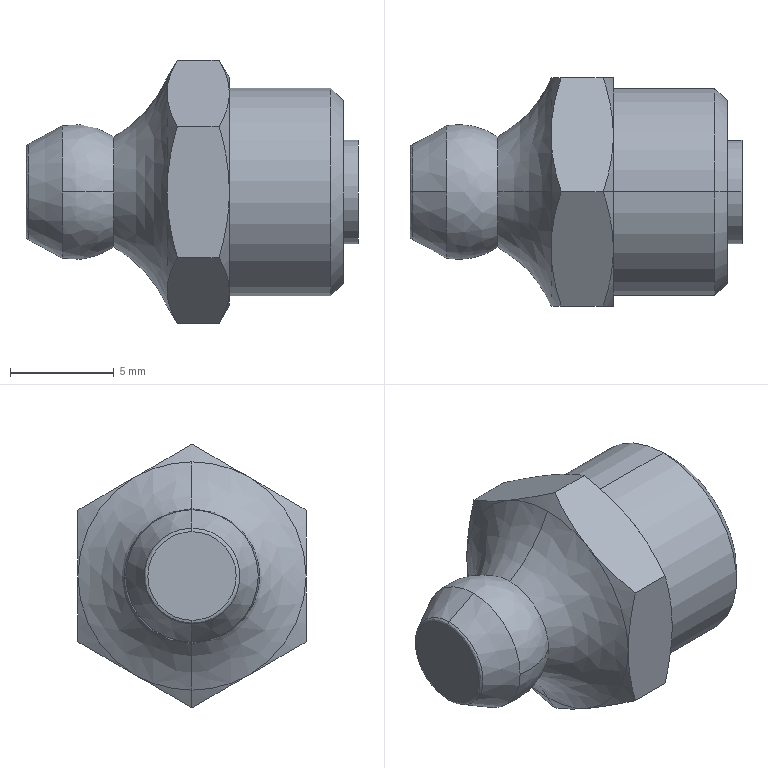Part | SolidWorks | features BaseBody 1 | 1 solid | 38 faces | box 16 x 11 x 12.702 mm | volume 986.989 mm3 | cone 18 | plane 10 | spline 6 | cylinder 4 | commonest cylinder face diameters 5 x2 10 x2
STEP:
#1=CARTESIAN_POINT('',(-5.573,0.,2.65));
#2=VERTEX_POINT('',#1);
#3=CARTESIAN_POINT('',(-5.573,2.65,0.));
#4=VERTEX_POINT('',#3);
#5=CARTESIAN_POINT('',(-5.573,0.,0.));
#6=DIRECTION('',(-1.,0.,0.));
#7=DIRECTION('',(0.,0.,-1.));
#8=AXIS2_PLACEMENT_3D('',#5,#6,#7);
#9=CIRCLE('',#8,2.65);
#10=EDGE_CURVE('',#2,#4,#9,.T.);
#11=ORIENTED_EDGE('',*,*,#10,.F.);
#12=CARTESIAN_POINT('',(-3.,0.,5.5));
#13=VERTEX_POINT('',#12);
#14=CARTESIAN_POINT('',(-8.506,0.,7.885));
#15=DIRECTION('',(0.,-1.,0.));
#16=DIRECTION('',(0.,0.,1.));
#17=AXIS2_PLACEMENT_3D('',#14,#15,#16);
#18=CIRCLE('',#17,6.);
#19=EDGE_CURVE('',#2,#13,#18,.T.);
#20=ORIENTED_EDGE('',*,*,#19,.T.);
#21=CARTESIAN_POINT('',(-3.,2.75,4.763));
#22=VERTEX_POINT('',#21);
#23=CARTESIAN_POINT('',(-3.,0.,0.));
#24=DIRECTION('',(1.,0.,0.));
#25=DIRECTION('',(0.,0.,1.));
#26=AXIS2_PLACEMENT_3D('',#23,#24,#25);
#27=CIRCLE('',#26,5.5);
#28=EDGE_CURVE('',#22,#13,#27,.T.);
#29=ORIENTED_EDGE('',*,*,#28,.F.);
#30=CARTESIAN_POINT('',(-3.,5.5,0.));
#31=VERTEX_POINT('',#30);
#32=CARTESIAN_POINT('',(-3.,0.,0.));
#33=DIRECTION('',(1.,0.,0.));
#34=DIRECTION('',(0.,0.,1.));
#35=AXIS2_PLACEMENT_3D('',#32,#33,#34);
#36=CIRCLE('',#35,5.5);
#37=EDGE_CURVE('',#31,#22,#36,.T.);
#38=ORIENTED_EDGE('',*,*,#37,.F.);
#39=CARTESIAN_POINT('',(-3.,2.75,-4.763));
#40=VERTEX_POINT('',#39);
#41=CARTESIAN_POINT('',(-3.,0.,0.));
#42=DIRECTION('',(1.,0.,0.));
#43=DIRECTION('',(0.,0.,1.));
#44=AXIS2_PLACEMENT_3D('',#41,#42,#43);
#45=CIRCLE('',#44,5.5);
#46=EDGE_CURVE('',#40,#31,#45,.T.);
#47=ORIENTED_EDGE('',*,*,#46,.F.);
#48=CARTESIAN_POINT('',(-3.,0.,-5.5));
#49=VERTEX_POINT('',#48);
#50=CARTESIAN_POINT('',(-3.,0.,0.));
#51=DIRECTION('',(1.,0.,0.));
#52=DIRECTION('',(0.,0.,1.));
#53=AXIS2_PLACEMENT_3D('',#50,#51,#52);
#54=CIRCLE('',#53,5.5);
#55=EDGE_CURVE('',#49,#40,#54,.T.);
#56=ORIENTED_EDGE('',*,*,#55,.F.);
#57=CARTESIAN_POINT('',(-5.573,0.,-2.65));
#58=VERTEX_POINT('',#57);
#59=CARTESIAN_POINT('',(-8.506,0.,-7.885));
#60=DIRECTION('',(0.,1.,0.));
#61=DIRECTION('',(0.,0.,-1.));
#62=AXIS2_PLACEMENT_3D('',#59,#60,#61);
#63=CIRCLE('',#62,6.);
#64=EDGE_CURVE('',#58,#49,#63,.T.);
#65=ORIENTED_EDGE('',*,*,#64,.F.);
#66=CARTESIAN_POINT('',(-5.573,0.,0.));
#67=DIRECTION('',(-1.,0.,0.));
#68=DIRECTION('',(0.,0.,-1.));
#69=AXIS2_PLACEMENT_3D('',#66,#67,#68);
#70=CIRCLE('',#69,2.65);
#71=EDGE_CURVE('',#4,#58,#70,.T.);
#72=ORIENTED_EDGE('',*,*,#71,.F.);
#73=EDGE_LOOP('',(#11,#20,#29,#38,#47,#56,#65,#72));
#74=FACE_OUTER_BOUND('',#73,.T.);
#75=CARTESIAN_POINT('',(-5.573,0.,-2.65));
#76=CARTESIAN_POINT('',(-5.573,5.3,-2.65));
#77=CARTESIAN_POINT('',(-5.573,5.3,2.65));
#78=CARTESIAN_POINT('',(-5.573,0.,2.65));
#79=CARTESIAN_POINT('',(-4.416,0.,-3.298));
#80=CARTESIAN_POINT('',(-4.416,6.597,-3.298));
#81=CARTESIAN_POINT('',(-4.416,6.597,3.298));
#82=CARTESIAN_POINT('',(-4.416,0.,3.298));
#83=CARTESIAN_POINT('',(-3.527,0.,-4.283));
#84=CARTESIAN_POINT('',(-3.527,8.566,-4.283));
#85=CARTESIAN_POINT('',(-3.527,8.566,4.283));
#86=CARTESIAN_POINT('',(-3.527,0.,4.283));
#87=CARTESIAN_POINT('',(-3.,0.,-5.5));
#88=CARTESIAN_POINT('',(-3.,11.,-5.5));
#89=CARTESIAN_POINT('',(-3.,11.,5.5));
#90=CARTESIAN_POINT('',(-3.,0.,5.5));
#91=(BOUNDED_SURFACE()B_SPLINE_SURFACE(3,3,((#75,#76,#77,#78),(#79,#80,#81,#82),(#83,#84,#85,#86),(#87,#88,#89,#90)),.UNSPECIFIED.,.F.,.F.,.T.)B_SPLINE_SURFACE_WITH_KNOTS((4,4),(4,4),(0.,1.),(0.,1.),.UNSPECIFIED.)GEOMETRIC_REPRESENTATION_ITEM()RATIONAL_B_SPLINE_SURFACE(((1.,0.3333,0.3333,1.),(0.9649,0.3216,0.3216,0.9649),(0.9649,0.3216,0.3216,0.9649),(1.,0.3333,0.3333,1.)))REPRESENTATION_ITEM('')SURFACE());
#92=ADVANCED_FACE('',(#74),#91,.F.);
#93=ORIENTED_EDGE('',*,*,#71,.T.);
#94=CARTESIAN_POINT('',(-5.573,-2.65,0.));
#95=VERTEX_POINT('',#94);
#96=CARTESIAN_POINT('',(-5.573,0.,0.));
#97=DIRECTION('',(-1.,0.,0.));
#98=DIRECTION('',(0.,0.,-1.));
#99=AXIS2_PLACEMENT_3D('',#96,#97,#98);
#100=CIRCLE('',#99,2.65);
#101=EDGE_CURVE('',#58,#95,#100,.T.);
#102=ORIENTED_EDGE('',*,*,#101,.T.);
#103=CARTESIAN_POINT('',(-8.055,-3.194,0.));
#104=VERTEX_POINT('',#103);
#105=CARTESIAN_POINT('',(-7.455,0.,0.));
#106=DIRECTION('',(0.,0.,-1.));
#107=DIRECTION('',(1.,0.,0.));
#108=AXIS2_PLACEMENT_3D('',#105,#106,#107);
#109=CIRCLE('',#108,3.25);
#110=EDGE_CURVE('',#95,#104,#109,.T.);
#111=ORIENTED_EDGE('',*,*,#110,.T.);
#112=CARTESIAN_POINT('',(-8.055,0.,-3.194));
#113=VERTEX_POINT('',#112);
#114=CARTESIAN_POINT('',(-8.055,0.,0.));
#115=DIRECTION('',(1.,0.,0.));
#116=DIRECTION('',(0.,1.,0.));
#117=AXIS2_PLACEMENT_3D('',#114,#115,#116);
#118=CIRCLE('',#117,3.194);
#119=EDGE_CURVE('',#104,#113,#118,.T.);
#120=ORIENTED_EDGE('',*,*,#119,.T.);
#121=CARTESIAN_POINT('',(-8.055,3.194,0.));
#122=VERTEX_POINT('',#121);
#123=CARTESIAN_POINT('',(-8.055,0.,0.));
#124=DIRECTION('',(1.,0.,0.));
#125=DIRECTION('',(0.,1.,0.));
#126=AXIS2_PLACEMENT_3D('',#123,#124,#125);
#127=CIRCLE('',#126,3.194);
#128=EDGE_CURVE('',#113,#122,#127,.T.);
#129=ORIENTED_EDGE('',*,*,#128,.T.);
#130=CARTESIAN_POINT('',(-7.455,0.,0.));
#131=DIRECTION('',(0.,0.,1.));
#132=DIRECTION('',(1.,0.,0.));
#133=AXIS2_PLACEMENT_3D('',#130,#131,#132);
#134=CIRCLE('',#133,3.25);
#135=EDGE_CURVE('',#4,#122,#134,.T.);
#136=ORIENTED_EDGE('',*,*,#135,.F.);
#137=EDGE_LOOP('',(#93,#102,#111,#120,#129,#136));
#138=FACE_OUTER_BOUND('',#137,.T.);
#139=CARTESIAN_POINT('',(-5.573,-2.65,0.));
#140=CARTESIAN_POINT('',(-5.573,-2.65,-5.3));
#141=CARTESIAN_POINT('',(-5.573,2.65,-5.3));
#142=CARTESIAN_POINT('',(-5.573,2.65,0.));
#143=CARTESIAN_POINT('',(-6.302,-3.168,0.));
#144=CARTESIAN_POINT('',(-6.302,-3.168,-6.335));
#145=CARTESIAN_POINT('',(-6.302,3.168,-6.335));
#146=CARTESIAN_POINT('',(-6.302,3.168,0.));
#147=CARTESIAN_POINT('',(-7.176,-3.359,0.));
#148=CARTESIAN_POINT('',(-7.176,-3.359,-6.718));
#149=CARTESIAN_POINT('',(-7.176,3.359,-6.718));
#150=CARTESIAN_POINT('',(-7.176,3.359,0.));
#151=CARTESIAN_POINT('',(-8.055,-3.194,0.));
#152=CARTESIAN_POINT('',(-8.055,-3.194,-6.388));
#153=CARTESIAN_POINT('',(-8.055,3.194,-6.388));
#154=CARTESIAN_POINT('',(-8.055,3.194,0.));
#155=(BOUNDED_SURFACE()B_SPLINE_SURFACE(3,3,((#139,#140,#141,#142),(#143,#144,#145,#146),(#147,#148,#149,#150),(#151,#152,#153,#154)),.UNSPECIFIED.,.F.,.F.,.F.)B_SPLINE_SURFACE_WITH_KNOTS((4,4),(4,4),(0.,1.),(0.,1.),.UNSPECIFIED.)GEOMETRIC_REPRESENTATION_ITEM()RATIONAL_B_SPLINE_SURFACE(((1.,0.3333,0.3333,1.),(0.947,0.3157,0.3157,0.947),(0.947,0.3157,0.3157,0.947),(1.,0.3333,0.3333,1.)))REPRESENTATION_ITEM('')SURFACE());
#156=ADVANCED_FACE('',(#138),#155,.T.);
#157=CARTESIAN_POINT('',(-9.695,0.,2.307));
#158=VERTEX_POINT('',#157);
#159=CARTESIAN_POINT('',(-9.695,0.,-2.307));
#160=VERTEX_POINT('',#159);
#161=CARTESIAN_POINT('',(-9.695,0.,0.));
#162=DIRECTION('',(1.,0.,0.));
#163=DIRECTION('',(0.,1.,0.));
#164=AXIS2_PLACEMENT_3D('',#161,#162,#163);
#165=CIRCLE('',#164,2.307);
#166=EDGE_CURVE('',#158,#160,#165,.T.);
#167=ORIENTED_EDGE('',*,*,#166,.F.);
#168=CARTESIAN_POINT('',(-9.8,0.,2.131));
#169=VERTEX_POINT('',#168);
#170=CARTESIAN_POINT('',(-9.6,0.,2.131));
#171=DIRECTION('',(0.,-1.,0.));
#172=DIRECTION('',(0.,0.,1.));
#173=AXIS2_PLACEMENT_3D('',#170,#171,#172);
#174=CIRCLE('',#173,0.2);
#175=EDGE_CURVE('',#158,#169,#174,.T.);
#176=ORIENTED_EDGE('',*,*,#175,.T.);
#177=CARTESIAN_POINT('',(-9.8,0.,-2.131));
#178=VERTEX_POINT('',#177);
#179=CARTESIAN_POINT('',(-9.8,0.,2.131));
#180=CARTESIAN_POINT('',(-9.8,-4.262,2.131));
#181=CARTESIAN_POINT('',(-9.8,-4.262,-2.131));
#182=CARTESIAN_POINT('',(-9.8,0.,-2.131));
#183=(BOUNDED_CURVE()B_SPLINE_CURVE(3,(#179,#180,#181,#182),.UNSPECIFIED.,.F.,.T.)B_SPLINE_CURVE_WITH_KNOTS((4,4),(0.25,0.75),.UNSPECIFIED.)CURVE()GEOMETRIC_REPRESENTATION_ITEM()RATIONAL_B_SPLINE_CURVE((1.,0.3333,0.3333,1.))REPRESENTATION_ITEM(''));
#184=EDGE_CURVE('',#169,#178,#183,.T.);
#185=ORIENTED_EDGE('',*,*,#184,.T.);
#186=CARTESIAN_POINT('',(-9.6,0.,-2.131));
#187=DIRECTION('',(0.,1.,0.));
#188=DIRECTION('',(0.,0.,-1.));
#189=AXIS2_PLACEMENT_3D('',#186,#187,#188);
#190=CIRCLE('',#189,0.2);
#191=EDGE_CURVE('',#160,#178,#190,.T.);
#192=ORIENTED_EDGE('',*,*,#191,.F.);
#193=EDGE_LOOP('',(#167,#176,#185,#192));
#194=FACE_OUTER_BOUND('',#193,.T.);
#195=CARTESIAN_POINT('',(-9.695,0.,2.307));
#196=CARTESIAN_POINT('',(-9.695,-4.613,2.307));
#197=CARTESIAN_POINT('',(-9.695,-4.613,-2.307));
#198=CARTESIAN_POINT('',(-9.695,0.,-2.307));
#199=CARTESIAN_POINT('',(-9.761,0.,2.271));
#200=CARTESIAN_POINT('',(-9.761,-4.542,2.271));
#201=CARTESIAN_POINT('',(-9.761,-4.542,-2.271));
#202=CARTESIAN_POINT('',(-9.761,0.,-2.271));
#203=CARTESIAN_POINT('',(-9.8,0.,2.206));
#204=CARTESIAN_POINT('',(-9.8,-4.412,2.206));
#205=CARTESIAN_POINT('',(-9.8,-4.412,-2.206));
#206=CARTESIAN_POINT('',(-9.8,0.,-2.206));
#207=CARTESIAN_POINT('',(-9.8,0.,2.131));
#208=CARTESIAN_POINT('',(-9.8,-4.262,2.131));
#209=CARTESIAN_POINT('',(-9.8,-4.262,-2.131));
#210=CARTESIAN_POINT('',(-9.8,0.,-2.131));
#211=(BOUNDED_SURFACE()B_SPLINE_SURFACE(3,3,((#195,#196,#197,#198),(#199,#200,#201,#202),(#203,#204,#205,#206),(#207,#208,#209,#210)),.UNSPECIFIED.,.F.,.F.,.F.)B_SPLINE_SURFACE_WITH_KNOTS((4,4),(4,4),(0.,1.),(0.,1.),.UNSPECIFIED.)GEOMETRIC_REPRESENTATION_ITEM()RATIONAL_B_SPLINE_SURFACE(((1.,0.3333,0.3333,1.),(0.906,0.302,0.302,0.906),(0.906,0.302,0.302,0.906),(1.,0.3333,0.3333,1.)))REPRESENTATION_ITEM('')SURFACE());
#212=ADVANCED_FACE('',(#194),#211,.T.);
#213=CARTESIAN_POINT('',(0.,0.,-5.));
#214=VERTEX_POINT('',#213);
#215=CARTESIAN_POINT('',(0.,0.,5.));
#216=VERTEX_POINT('',#215);
#217=CARTESIAN_POINT('',(0.,0.,0.));
#218=DIRECTION('',(1.,0.,0.));
#219=DIRECTION('',(0.,0.,-1.));
#220=AXIS2_PLACEMENT_3D('',#217,#218,#219);
#221=CIRCLE('',#220,5.);
#222=EDGE_CURVE('',#214,#216,#221,.T.);
#223=ORIENTED_EDGE('',*,*,#222,.T.);
#224=CARTESIAN_POINT('',(4.887,0.,5.));
#225=VERTEX_POINT('',#224);
#226=CARTESIAN_POINT('',(2.75,0.,5.));
#227=DIRECTION('',(1.,0.,0.));
#228=VECTOR('',#227,1000.);
#229=LINE('',#226,#228);
#230=EDGE_CURVE('',#216,#225,#229,.T.);
#231=ORIENTED_EDGE('',*,*,#230,.T.);
#232=CARTESIAN_POINT('',(4.887,0.,-5.));
#233=VERTEX_POINT('',#232);
#234=CARTESIAN_POINT('',(4.887,0.,0.));
#235=DIRECTION('',(-1.,0.,0.));
#236=DIRECTION('',(0.,0.,-1.));
#237=AXIS2_PLACEMENT_3D('',#234,#235,#236);
#238=CIRCLE('',#237,5.);
#239=EDGE_CURVE('',#225,#233,#238,.T.);
#240=ORIENTED_EDGE('',*,*,#239,.T.);
#241=CARTESIAN_POINT('',(2.75,0.,-5.));
#242=DIRECTION('',(1.,0.,0.));
#243=VECTOR('',#242,1000.);
#244=LINE('',#241,#243);
#245=EDGE_CURVE('',#214,#233,#244,.T.);
#246=ORIENTED_EDGE('',*,*,#245,.F.);
#247=EDGE_LOOP('',(#223,#231,#240,#246));
#248=FACE_OUTER_BOUND('',#247,.T.);
#249=CARTESIAN_POINT('',(2.75,0.,0.));
#250=DIRECTION('',(1.,0.,0.));
#251=DIRECTION('',(0.,0.,-1.));
#252=AXIS2_PLACEMENT_3D('',#249,#250,#251);
#253=CYLINDRICAL_SURFACE('',#252,5.);
#254=ADVANCED_FACE('',(#248),#253,.T.);
#255=CARTESIAN_POINT('',(5.5,0.,4.387));
#256=VERTEX_POINT('',#255);
#257=CARTESIAN_POINT('',(5.5,0.,-4.387));
#258=VERTEX_POINT('',#257);
#259=CARTESIAN_POINT('',(5.5,0.,0.));
#260=DIRECTION('',(-1.,0.,0.));
#261=DIRECTION('',(0.,0.,1.));
#262=AXIS2_PLACEMENT_3D('',#259,#260,#261);
#263=CIRCLE('',#262,4.387);
#264=EDGE_CURVE('',#256,#258,#263,.T.);
#265=ORIENTED_EDGE('',*,*,#264,.T.);
#266=CARTESIAN_POINT('',(4.887,0.,-5.));
#267=DIRECTION('',(-0.7071,0.,-0.7071));
#268=VECTOR('',#267,1000.);
#269=LINE('',#266,#268);
#270=EDGE_CURVE('',#258,#233,#269,.T.);
#271=ORIENTED_EDGE('',*,*,#270,.T.);
#272=ORIENTED_EDGE('',*,*,#239,.F.);
#273=CARTESIAN_POINT('',(4.887,0.,5.));
#274=DIRECTION('',(-0.7071,0.,0.7071));
#275=VECTOR('',#274,1000.);
#276=LINE('',#273,#275);
#277=EDGE_CURVE('',#256,#225,#276,.T.);
#278=ORIENTED_EDGE('',*,*,#277,.F.);
#279=EDGE_LOOP('',(#265,#271,#272,#278));
#280=FACE_OUTER_BOUND('',#279,.T.);
#281=CARTESIAN_POINT('',(4.887,0.,0.));
#282=DIRECTION('',(-1.,0.,0.));
#283=DIRECTION('',(0.,0.,1.));
#284=AXIS2_PLACEMENT_3D('',#281,#282,#283);
#285=CONICAL_SURFACE('',#284,5.,0.7854);
#286=ADVANCED_FACE('',(#280),#285,.T.);
#287=CARTESIAN_POINT('',(0.,0.,5.5));
#288=VERTEX_POINT('',#287);
#289=CARTESIAN_POINT('',(0.,-2.75,4.763));
#290=VERTEX_POINT('',#289);
#291=CARTESIAN_POINT('',(0.,0.,0.));
#292=DIRECTION('',(1.,0.,0.));
#293=DIRECTION('',(0.,0.,1.));
#294=AXIS2_PLACEMENT_3D('',#291,#292,#293);
#295=CIRCLE('',#294,5.5);
#296=EDGE_CURVE('',#288,#290,#295,.T.);
#297=ORIENTED_EDGE('',*,*,#296,.F.);
#298=CARTESIAN_POINT('',(-0.4912,-0.000000012,6.351));
#299=VERTEX_POINT('',#298);
#300=CARTESIAN_POINT('',(-0.4942,0.,6.356));
#301=DIRECTION('',(-0.5,0.,0.866));
#302=VECTOR('',#301,1000.);
#303=LINE('',#300,#302);
#304=EDGE_CURVE('',#288,#299,#303,.T.);
#305=ORIENTED_EDGE('',*,*,#304,.T.);
#306=CARTESIAN_POINT('',(-0.4912,-0.000000012,6.351));
#307=CARTESIAN_POINT('',(-0.1917,-0.8985,5.832));
#308=CARTESIAN_POINT('',(0.,-1.811,5.305));
#309=CARTESIAN_POINT('',(0.,-2.75,4.763));
#310=B_SPLINE_CURVE_WITH_KNOTS('',3,(#306,#307,#308,#309),.UNSPECIFIED.,.F.,.F.,(4,4),(0.,0.003213),.UNSPECIFIED.);
#311=EDGE_CURVE('',#299,#290,#310,.T.);
#312=ORIENTED_EDGE('',*,*,#311,.T.);
#313=EDGE_LOOP('',(#297,#305,#312));
#314=FACE_OUTER_BOUND('',#313,.T.);
#315=CARTESIAN_POINT('',(-0.4942,0.,0.));
#316=DIRECTION('',(-1.,0.,0.));
#317=DIRECTION('',(0.,0.,1.));
#318=AXIS2_PLACEMENT_3D('',#315,#316,#317);
#319=CONICAL_SURFACE('',#318,6.356,1.047);
#320=ADVANCED_FACE('',(#314),#319,.T.);
#321=CARTESIAN_POINT('',(5.5,0.,2.5));
#322=VERTEX_POINT('',#321);
#323=CARTESIAN_POINT('',(5.5,0.,-2.5));
#324=VERTEX_POINT('',#323);
#325=CARTESIAN_POINT('',(5.5,0.,0.));
#326=DIRECTION('',(-1.,0.,0.));
#327=DIRECTION('',(0.,0.,-1.));
#328=AXIS2_PLACEMENT_3D('',#325,#326,#327);
#329=CIRCLE('',#328,2.5);
#330=EDGE_CURVE('',#322,#324,#329,.T.);
#331=ORIENTED_EDGE('',*,*,#330,.F.);
#332=CARTESIAN_POINT('',(6.2,0.,2.5));
#333=VERTEX_POINT('',#332);
#334=CARTESIAN_POINT('',(5.85,0.,2.5));
#335=DIRECTION('',(1.,0.,0.));
#336=VECTOR('',#335,1000.);
#337=LINE('',#334,#336);
#338=EDGE_CURVE('',#322,#333,#337,.T.);
#339=ORIENTED_EDGE('',*,*,#338,.T.);
#340=CARTESIAN_POINT('',(6.2,0.,-2.5));
#341=VERTEX_POINT('',#340);
#342=CARTESIAN_POINT('',(6.2,0.,0.));
#343=DIRECTION('',(-1.,0.,0.));
#344=DIRECTION('',(0.,0.,-1.));
#345=AXIS2_PLACEMENT_3D('',#342,#343,#344);
#346=CIRCLE('',#345,2.5);
#347=EDGE_CURVE('',#333,#341,#346,.T.);
#348=ORIENTED_EDGE('',*,*,#347,.T.);
#349=CARTESIAN_POINT('',(5.85,0.,-2.5));
#350=DIRECTION('',(1.,0.,0.));
#351=VECTOR('',#350,1000.);
#352=LINE('',#349,#351);
#353=EDGE_CURVE('',#324,#341,#352,.T.);
#354=ORIENTED_EDGE('',*,*,#353,.F.);
#355=EDGE_LOOP('',(#331,#339,#348,#354));
#356=FACE_OUTER_BOUND('',#355,.T.);
#357=CARTESIAN_POINT('',(5.85,0.,0.));
#358=DIRECTION('',(1.,0.,0.));
#359=DIRECTION('',(0.,0.,-1.));
#360=AXIS2_PLACEMENT_3D('',#357,#358,#359);
#361=CYLINDRICAL_SURFACE('',#360,2.5);
#362=ADVANCED_FACE('',(#356),#361,.T.);
#363=CARTESIAN_POINT('',(-3.,-2.75,-4.763));
#364=VERTEX_POINT('',#363);
#365=CARTESIAN_POINT('',(-3.,0.,0.));
#366=DIRECTION('',(1.,0.,0.));
#367=DIRECTION('',(0.,0.,1.));
#368=AXIS2_PLACEMENT_3D('',#365,#366,#367);
#369=CIRCLE('',#368,5.5);
#370=EDGE_CURVE('',#364,#49,#369,.T.);
#371=ORIENTED_EDGE('',*,*,#370,.T.);
#372=CARTESIAN_POINT('',(-2.509,0.,-6.351));
#373=VERTEX_POINT('',#372);
#374=CARTESIAN_POINT('',(-2.506,0.,-6.356));
#375=DIRECTION('',(0.5,0.,-0.866));
#376=VECTOR('',#375,1000.);
#377=LINE('',#374,#376);
#378=EDGE_CURVE('',#49,#373,#377,.T.);
#379=ORIENTED_EDGE('',*,*,#378,.T.);
#380=CARTESIAN_POINT('',(-3.,-2.75,-4.763));
#381=CARTESIAN_POINT('',(-3.,-1.811,-5.305));
#382=CARTESIAN_POINT('',(-2.808,-0.8985,-5.832));
#383=CARTESIAN_POINT('',(-2.509,0.,-6.351));
#384=B_SPLINE_CURVE_WITH_KNOTS('',3,(#380,#381,#382,#383),.UNSPECIFIED.,.F.,.F.,(4,4),(0.,0.003213),.UNSPECIFIED.);
#385=EDGE_CURVE('',#364,#373,#384,.T.);
#386=ORIENTED_EDGE('',*,*,#385,.F.);
#387=EDGE_LOOP('',(#371,#379,#386));
#388=FACE_OUTER_BOUND('',#387,.T.);
#389=CARTESIAN_POINT('',(-2.506,0.,0.));
#390=DIRECTION('',(1.,0.,0.));
#391=DIRECTION('',(0.,0.,-1.));
#392=AXIS2_PLACEMENT_3D('',#389,#390,#391);
#393=CONICAL_SURFACE('',#392,6.356,1.047);
#394=ADVANCED_FACE('',(#388),#393,.T.);
#395=CARTESIAN_POINT('',(-9.695,0.,0.));
#396=DIRECTION('',(1.,0.,0.));
#397=DIRECTION('',(0.,1.,0.));
#398=AXIS2_PLACEMENT_3D('',#395,#396,#397);
#399=CIRCLE('',#398,2.307);
#400=EDGE_CURVE('',#160,#158,#399,.T.);
#401=ORIENTED_EDGE('',*,*,#400,.T.);
#402=CARTESIAN_POINT('',(-8.055,0.,3.194));
#403=VERTEX_POINT('',#402);
#404=CARTESIAN_POINT('',(-8.055,0.,3.194));
#405=DIRECTION('',(0.8795,0.,0.4758));
#406=VECTOR('',#405,1000.);
#407=LINE('',#404,#406);
#408=EDGE_CURVE('',#158,#403,#407,.T.);
#409=ORIENTED_EDGE('',*,*,#408,.T.);
#410=CARTESIAN_POINT('',(-8.055,0.,0.));
#411=DIRECTION('',(1.,0.,0.));
#412=DIRECTION('',(0.,1.,0.));
#413=AXIS2_PLACEMENT_3D('',#410,#411,#412);
#414=CIRCLE('',#413,3.194);
#415=EDGE_CURVE('',#122,#403,#414,.T.);
#416=ORIENTED_EDGE('',*,*,#415,.F.);
#417=ORIENTED_EDGE('',*,*,#128,.F.);
#418=CARTESIAN_POINT('',(-8.055,0.,-3.194));
#419=DIRECTION('',(0.8795,0.,-0.4758));
#420=VECTOR('',#419,1000.);
#421=LINE('',#418,#420);
#422=EDGE_CURVE('',#160,#113,#421,.T.);
#423=ORIENTED_EDGE('',*,*,#422,.F.);
#424=EDGE_LOOP('',(#401,#409,#416,#417,#423));
#425=FACE_OUTER_BOUND('',#424,.T.);
#426=CARTESIAN_POINT('',(-8.055,0.,0.));
#427=DIRECTION('',(1.,0.,0.));
#428=DIRECTION('',(0.,0.,-1.));
#429=AXIS2_PLACEMENT_3D('',#426,#427,#428);
#430=CONICAL_SURFACE('',#429,3.194,0.4959);
#431=ADVANCED_FACE('',(#425),#430,.T.);
#432=ORIENTED_EDGE('',*,*,#230,.F.);
#433=CARTESIAN_POINT('',(0.,0.,0.));
#434=DIRECTION('',(1.,0.,0.));
#435=DIRECTION('',(0.,0.,-1.));
#436=AXIS2_PLACEMENT_3D('',#433,#434,#435);
#437=CIRCLE('',#436,5.);
#438=EDGE_CURVE('',#216,#214,#437,.T.);
#439=ORIENTED_EDGE('',*,*,#438,.T.);
#440=ORIENTED_EDGE('',*,*,#245,.T.);
#441=CARTESIAN_POINT('',(4.887,0.,0.));
#442=DIRECTION('',(-1.,0.,0.));
#443=DIRECTION('',(0.,0.,-1.));
#444=AXIS2_PLACEMENT_3D('',#441,#442,#443);
#445=CIRCLE('',#444,5.);
#446=EDGE_CURVE('',#233,#225,#445,.T.);
#447=ORIENTED_EDGE('',*,*,#446,.T.);
#448=EDGE_LOOP('',(#432,#439,#440,#447));
#449=FACE_OUTER_BOUND('',#448,.T.);
#450=CARTESIAN_POINT('',(2.75,0.,0.));
#451=DIRECTION('',(1.,0.,0.));
#452=DIRECTION('',(0.,0.,-1.));
#453=AXIS2_PLACEMENT_3D('',#450,#451,#452);
#454=CYLINDRICAL_SURFACE('',#453,5.);
#455=ADVANCED_FACE('',(#449),#454,.T.);
#456=ORIENTED_EDGE('',*,*,#270,.F.);
#457=CARTESIAN_POINT('',(5.5,0.,0.));
#458=DIRECTION('',(-1.,0.,0.));
#459=DIRECTION('',(0.,0.,1.));
#460=AXIS2_PLACEMENT_3D('',#457,#458,#459);
#461=CIRCLE('',#460,4.387);
#462=EDGE_CURVE('',#258,#256,#461,.T.);
#463=ORIENTED_EDGE('',*,*,#462,.T.);
#464=ORIENTED_EDGE('',*,*,#277,.T.);
#465=ORIENTED_EDGE('',*,*,#446,.F.);
#466=EDGE_LOOP('',(#456,#463,#464,#465));
#467=FACE_OUTER_BOUND('',#466,.T.);
#468=CARTESIAN_POINT('',(4.887,0.,0.));
#469=DIRECTION('',(-1.,0.,0.));
#470=DIRECTION('',(0.,0.,1.));
#471=AXIS2_PLACEMENT_3D('',#468,#469,#470);
#472=CONICAL_SURFACE('',#471,5.,0.7854);
#473=ADVANCED_FACE('',(#467),#472,.T.);
#474=ORIENTED_EDGE('',*,*,#222,.F.);
#475=ORIENTED_EDGE('',*,*,#438,.F.);
#476=EDGE_LOOP('',(#474,#475));
#477=FACE_BOUND('',#476,.T.);
#478=CARTESIAN_POINT('',(0.,-2.75,-4.763));
#479=VERTEX_POINT('',#478);
#480=CARTESIAN_POINT('',(0.,2.75,-4.763));
#481=VERTEX_POINT('',#480);
#482=CARTESIAN_POINT('',(0.,0.,0.));
#483=DIRECTION('',(1.,0.,0.));
#484=DIRECTION('',(0.,0.,1.));
#485=AXIS2_PLACEMENT_3D('',#482,#483,#484);
#486=CIRCLE('',#485,5.5);
#487=EDGE_CURVE('',#479,#481,#486,.T.);
#488=ORIENTED_EDGE('',*,*,#487,.T.);
#489=CARTESIAN_POINT('',(0.,5.5,0.));
#490=VERTEX_POINT('',#489);
#491=CARTESIAN_POINT('',(0.,0.,0.));
#492=DIRECTION('',(1.,0.,0.));
#493=DIRECTION('',(0.,0.,1.));
#494=AXIS2_PLACEMENT_3D('',#491,#492,#493);
#495=CIRCLE('',#494,5.5);
#496=EDGE_CURVE('',#481,#490,#495,.T.);
#497=ORIENTED_EDGE('',*,*,#496,.T.);
#498=CARTESIAN_POINT('',(0.,2.75,4.763));
#499=VERTEX_POINT('',#498);
#500=CARTESIAN_POINT('',(0.,0.,0.));
#501=DIRECTION('',(1.,0.,0.));
#502=DIRECTION('',(0.,0.,1.));
#503=AXIS2_PLACEMENT_3D('',#500,#501,#502);
#504=CIRCLE('',#503,5.5);
#505=EDGE_CURVE('',#490,#499,#504,.T.);
#506=ORIENTED_EDGE('',*,*,#505,.T.);
#507=CARTESIAN_POINT('',(0.,0.,0.));
#508=DIRECTION('',(1.,0.,0.));
#509=DIRECTION('',(0.,0.,1.));
#510=AXIS2_PLACEMENT_3D('',#507,#508,#509);
#511=CIRCLE('',#510,5.5);
#512=EDGE_CURVE('',#499,#288,#511,.T.);
#513=ORIENTED_EDGE('',*,*,#512,.T.);
#514=ORIENTED_EDGE('',*,*,#296,.T.);
#515=CARTESIAN_POINT('',(0.,-5.5,0.));
#516=VERTEX_POINT('',#515);
#517=CARTESIAN_POINT('',(0.,0.,0.));
#518=DIRECTION('',(1.,0.,0.));
#519=DIRECTION('',(0.,0.,1.));
#520=AXIS2_PLACEMENT_3D('',#517,#518,#519);
#521=CIRCLE('',#520,5.5);
#522=EDGE_CURVE('',#290,#516,#521,.T.);
#523=ORIENTED_EDGE('',*,*,#522,.T.);
#524=CARTESIAN_POINT('',(0.,0.,0.));
#525=DIRECTION('',(1.,0.,0.));
#526=DIRECTION('',(0.,0.,1.));
#527=AXIS2_PLACEMENT_3D('',#524,#525,#526);
#528=CIRCLE('',#527,5.5);
#529=EDGE_CURVE('',#516,#479,#528,.T.);
#530=ORIENTED_EDGE('',*,*,#529,.T.);
#531=EDGE_LOOP('',(#488,#497,#506,#513,#514,#523,#530));
#532=FACE_OUTER_BOUND('',#531,.T.);
#533=CARTESIAN_POINT('',(0.,5.25,0.));
#534=DIRECTION('',(1.,0.,0.));
#535=DIRECTION('',(0.,0.,-1.));
#536=AXIS2_PLACEMENT_3D('',#533,#534,#535);
#537=PLANE('',#536);
#538=ADVANCED_FACE('',(#477,#532),#537,.T.);
#539=CARTESIAN_POINT('',(5.5,0.,0.));
#540=DIRECTION('',(-1.,0.,0.));
#541=DIRECTION('',(0.,0.,-1.));
#542=AXIS2_PLACEMENT_3D('',#539,#540,#541);
#543=CIRCLE('',#542,2.5);
#544=EDGE_CURVE('',#324,#322,#543,.T.);
#545=ORIENTED_EDGE('',*,*,#544,.T.);
#546=ORIENTED_EDGE('',*,*,#330,.T.);
#547=EDGE_LOOP('',(#545,#546));
#548=FACE_BOUND('',#547,.T.);
#549=ORIENTED_EDGE('',*,*,#264,.F.);
#550=ORIENTED_EDGE('',*,*,#462,.F.);
#551=EDGE_LOOP('',(#549,#550));
#552=FACE_OUTER_BOUND('',#551,.T.);
#553=CARTESIAN_POINT('',(5.5,3.75,0.));
#554=DIRECTION('',(1.,0.,0.));
#555=DIRECTION('',(0.,0.,-1.));
#556=AXIS2_PLACEMENT_3D('',#553,#554,#555);
#557=PLANE('',#556);
#558=ADVANCED_FACE('',(#548,#552),#557,.T.);
#559=CARTESIAN_POINT('',(-0.4912,5.5,-3.175));
#560=VERTEX_POINT('',#559);
#561=CARTESIAN_POINT('',(-0.4912,5.5,-3.175));
#562=CARTESIAN_POINT('',(-0.1917,5.5,-2.138));
#563=CARTESIAN_POINT('',(0.,5.5,-1.084));
#564=CARTESIAN_POINT('',(0.,5.5,0.));
#565=B_SPLINE_CURVE_WITH_KNOTS('',3,(#561,#562,#563,#564),.UNSPECIFIED.,.F.,.F.,(4,4),(0.,0.003213),.UNSPECIFIED.);
#566=EDGE_CURVE('',#560,#490,#565,.T.);
#567=ORIENTED_EDGE('',*,*,#566,.T.);
#568=ORIENTED_EDGE('',*,*,#496,.F.);
#569=CARTESIAN_POINT('',(0.,2.75,-4.763));
#570=CARTESIAN_POINT('',(0.,3.689,-4.221));
#571=CARTESIAN_POINT('',(-0.1917,4.602,-3.694));
#572=CARTESIAN_POINT('',(-0.4912,5.5,-3.175));
#573=B_SPLINE_CURVE_WITH_KNOTS('',3,(#569,#570,#571,#572),.UNSPECIFIED.,.F.,.F.,(4,4),(0.,0.003213),.UNSPECIFIED.);
#574=EDGE_CURVE('',#481,#560,#573,.T.);
#575=ORIENTED_EDGE('',*,*,#574,.T.);
#576=EDGE_LOOP('',(#567,#568,#575));
#577=FACE_OUTER_BOUND('',#576,.T.);
#578=CARTESIAN_POINT('',(-0.4942,0.,0.));
#579=DIRECTION('',(-1.,0.,0.));
#580=DIRECTION('',(0.,0.,1.));
#581=AXIS2_PLACEMENT_3D('',#578,#579,#580);
#582=CONICAL_SURFACE('',#581,6.356,1.047);
#583=ADVANCED_FACE('',(#577),#582,.T.);
#584=CARTESIAN_POINT('',(-0.4912,-0.000000014,-6.351));
#585=VERTEX_POINT('',#584);
#586=CARTESIAN_POINT('',(-0.4912,-0.000000014,-6.351));
#587=CARTESIAN_POINT('',(-0.1917,0.8985,-5.832));
#588=CARTESIAN_POINT('',(0.,1.811,-5.305));
#589=CARTESIAN_POINT('',(0.,2.75,-4.763));
#590=B_SPLINE_CURVE_WITH_KNOTS('',3,(#586,#587,#588,#589),.UNSPECIFIED.,.F.,.F.,(4,4),(0.,0.003213),.UNSPECIFIED.);
#591=EDGE_CURVE('',#585,#481,#590,.T.);
#592=ORIENTED_EDGE('',*,*,#591,.T.);
#593=ORIENTED_EDGE('',*,*,#487,.F.);
#594=CARTESIAN_POINT('',(0.,-2.75,-4.763));
#595=CARTESIAN_POINT('',(0.,-1.811,-5.305));
#596=CARTESIAN_POINT('',(-0.1917,-0.8985,-5.832));
#597=CARTESIAN_POINT('',(-0.4912,-0.000000014,-6.351));
#598=B_SPLINE_CURVE_WITH_KNOTS('',3,(#594,#595,#596,#597),.UNSPECIFIED.,.F.,.F.,(4,4),(0.,0.003213),.UNSPECIFIED.);
#599=EDGE_CURVE('',#479,#585,#598,.T.);
#600=ORIENTED_EDGE('',*,*,#599,.T.);
#601=EDGE_LOOP('',(#592,#593,#600));
#602=FACE_OUTER_BOUND('',#601,.T.);
#603=CARTESIAN_POINT('',(-0.4942,0.,0.));
#604=DIRECTION('',(-1.,0.,0.));
#605=DIRECTION('',(0.,0.,1.));
#606=AXIS2_PLACEMENT_3D('',#603,#604,#605);
#607=CONICAL_SURFACE('',#606,6.356,1.047);
#608=ADVANCED_FACE('',(#602),#607,.T.);
#609=CARTESIAN_POINT('',(-0.4912,-5.5,-3.175));
#610=VERTEX_POINT('',#609);
#611=CARTESIAN_POINT('',(-0.4912,-5.5,-3.175));
#612=CARTESIAN_POINT('',(-0.1917,-4.602,-3.694));
#613=CARTESIAN_POINT('',(0.,-3.689,-4.221));
#614=CARTESIAN_POINT('',(0.,-2.75,-4.763));
#615=B_SPLINE_CURVE_WITH_KNOTS('',3,(#611,#612,#613,#614),.UNSPECIFIED.,.F.,.F.,(4,4),(0.,0.003213),.UNSPECIFIED.);
#616=EDGE_CURVE('',#610,#479,#615,.T.);
#617=ORIENTED_EDGE('',*,*,#616,.T.);
#618=ORIENTED_EDGE('',*,*,#529,.F.);
#619=CARTESIAN_POINT('',(0.,-5.5,0.));
#620=CARTESIAN_POINT('',(0.,-5.5,-1.084));
#621=CARTESIAN_POINT('',(-0.1917,-5.5,-2.138));
#622=CARTESIAN_POINT('',(-0.4912,-5.5,-3.175));
#623=B_SPLINE_CURVE_WITH_KNOTS('',3,(#619,#620,#621,#622),.UNSPECIFIED.,.F.,.F.,(4,4),(0.,0.003213),.UNSPECIFIED.);
#624=EDGE_CURVE('',#516,#610,#623,.T.);
#625=ORIENTED_EDGE('',*,*,#624,.T.);
#626=EDGE_LOOP('',(#617,#618,#625));
#627=FACE_OUTER_BOUND('',#626,.T.);
#628=CARTESIAN_POINT('',(-0.4942,0.,0.));
#629=DIRECTION('',(-1.,0.,0.));
#630=DIRECTION('',(0.,0.,1.));
#631=AXIS2_PLACEMENT_3D('',#628,#629,#630);
#632=CONICAL_SURFACE('',#631,6.356,1.047);
#633=ADVANCED_FACE('',(#627),#632,.T.);
#634=ORIENTED_EDGE('',*,*,#522,.F.);
#635=CARTESIAN_POINT('',(-0.4912,-5.5,3.175));
#636=VERTEX_POINT('',#635);
#637=CARTESIAN_POINT('',(0.,-2.75,4.763));
#638=CARTESIAN_POINT('',(0.,-3.689,4.221));
#639=CARTESIAN_POINT('',(-0.1917,-4.602,3.694));
#640=CARTESIAN_POINT('',(-0.4912,-5.5,3.175));
#641=B_SPLINE_CURVE_WITH_KNOTS('',3,(#637,#638,#639,#640),.UNSPECIFIED.,.F.,.F.,(4,4),(0.,0.003213),.UNSPECIFIED.);
#642=EDGE_CURVE('',#290,#636,#641,.T.);
#643=ORIENTED_EDGE('',*,*,#642,.T.);
#644=CARTESIAN_POINT('',(-0.4912,-5.5,3.175));
#645=CARTESIAN_POINT('',(-0.1917,-5.5,2.138));
#646=CARTESIAN_POINT('',(0.,-5.5,1.084));
#647=CARTESIAN_POINT('',(0.,-5.5,0.));
#648=B_SPLINE_CURVE_WITH_KNOTS('',3,(#644,#645,#646,#647),.UNSPECIFIED.,.F.,.F.,(4,4),(0.,0.003213),.UNSPECIFIED.);
#649=EDGE_CURVE('',#636,#516,#648,.T.);
#650=ORIENTED_EDGE('',*,*,#649,.T.);
#651=EDGE_LOOP('',(#634,#643,#650));
#652=FACE_OUTER_BOUND('',#651,.T.);
#653=CARTESIAN_POINT('',(-0.4942,0.,0.));
#654=DIRECTION('',(-1.,0.,0.));
#655=DIRECTION('',(0.,0.,1.));
#656=AXIS2_PLACEMENT_3D('',#653,#654,#655);
#657=CONICAL_SURFACE('',#656,6.356,1.047);
#658=ADVANCED_FACE('',(#652),#657,.T.);
#659=ORIENTED_EDGE('',*,*,#304,.F.);
#660=ORIENTED_EDGE('',*,*,#512,.F.);
#661=CARTESIAN_POINT('',(0.,2.75,4.763));
#662=CARTESIAN_POINT('',(0.,1.811,5.305));
#663=CARTESIAN_POINT('',(-0.1917,0.8985,5.832));
#664=CARTESIAN_POINT('',(-0.4912,-0.000000012,6.351));
#665=B_SPLINE_CURVE_WITH_KNOTS('',3,(#661,#662,#663,#664),.UNSPECIFIED.,.F.,.F.,(4,4),(0.,0.003213),.UNSPECIFIED.);
#666=EDGE_CURVE('',#499,#299,#665,.T.);
#667=ORIENTED_EDGE('',*,*,#666,.T.);
#668=EDGE_LOOP('',(#659,#660,#667));
#669=FACE_OUTER_BOUND('',#668,.T.);
#670=CARTESIAN_POINT('',(-0.4942,0.,0.));
#671=DIRECTION('',(-1.,0.,0.));
#672=DIRECTION('',(0.,0.,1.));
#673=AXIS2_PLACEMENT_3D('',#670,#671,#672);
#674=CONICAL_SURFACE('',#673,6.356,1.047);
#675=ADVANCED_FACE('',(#669),#674,.T.);
#676=ORIENTED_EDGE('',*,*,#505,.F.);
#677=CARTESIAN_POINT('',(-0.4912,5.5,3.175));
#678=VERTEX_POINT('',#677);
#679=CARTESIAN_POINT('',(0.,5.5,0.));
#680=CARTESIAN_POINT('',(0.,5.5,1.084));
#681=CARTESIAN_POINT('',(-0.1917,5.5,2.138));
#682=CARTESIAN_POINT('',(-0.4912,5.5,3.175));
#683=B_SPLINE_CURVE_WITH_KNOTS('',3,(#679,#680,#681,#682),.UNSPECIFIED.,.F.,.F.,(4,4),(0.,0.003213),.UNSPECIFIED.);
#684=EDGE_CURVE('',#490,#678,#683,.T.);
#685=ORIENTED_EDGE('',*,*,#684,.T.);
#686=CARTESIAN_POINT('',(-0.4912,5.5,3.175));
#687=CARTESIAN_POINT('',(-0.1917,4.602,3.694));
#688=CARTESIAN_POINT('',(0.,3.689,4.221));
#689=CARTESIAN_POINT('',(0.,2.75,4.763));
#690=B_SPLINE_CURVE_WITH_KNOTS('',3,(#686,#687,#688,#689),.UNSPECIFIED.,.F.,.F.,(4,4),(0.,0.003213),.UNSPECIFIED.);
#691=EDGE_CURVE('',#678,#499,#690,.T.);
#692=ORIENTED_EDGE('',*,*,#691,.T.);
#693=EDGE_LOOP('',(#676,#685,#692));
#694=FACE_OUTER_BOUND('',#693,.T.);
#695=CARTESIAN_POINT('',(-0.4942,0.,0.));
#696=DIRECTION('',(-1.,0.,0.));
#697=DIRECTION('',(0.,0.,1.));
#698=AXIS2_PLACEMENT_3D('',#695,#696,#697);
#699=CONICAL_SURFACE('',#698,6.356,1.047);
#700=ADVANCED_FACE('',(#694),#699,.T.);
#701=ORIENTED_EDGE('',*,*,#338,.F.);
#702=ORIENTED_EDGE('',*,*,#544,.F.);
#703=ORIENTED_EDGE('',*,*,#353,.T.);
#704=CARTESIAN_POINT('',(6.2,0.,0.));
#705=DIRECTION('',(-1.,0.,0.));
#706=DIRECTION('',(0.,0.,-1.));
#707=AXIS2_PLACEMENT_3D('',#704,#705,#706);
#708=CIRCLE('',#707,2.5);
#709=EDGE_CURVE('',#341,#333,#708,.T.);
#710=ORIENTED_EDGE('',*,*,#709,.T.);
#711=EDGE_LOOP('',(#701,#702,#703,#710));
#712=FACE_OUTER_BOUND('',#711,.T.);
#713=CARTESIAN_POINT('',(5.85,0.,0.));
#714=DIRECTION('',(1.,0.,0.));
#715=DIRECTION('',(0.,0.,-1.));
#716=AXIS2_PLACEMENT_3D('',#713,#714,#715);
#717=CYLINDRICAL_SURFACE('',#716,2.5);
#718=ADVANCED_FACE('',(#712),#717,.T.);
#719=CARTESIAN_POINT('',(-2.509,5.5,3.175));
#720=VERTEX_POINT('',#719);
#721=CARTESIAN_POINT('',(-3.,5.5,0.));
#722=CARTESIAN_POINT('',(-3.,5.5,1.084));
#723=CARTESIAN_POINT('',(-2.808,5.5,2.138));
#724=CARTESIAN_POINT('',(-2.509,5.5,3.175));
#725=B_SPLINE_CURVE_WITH_KNOTS('',3,(#721,#722,#723,#724),.UNSPECIFIED.,.F.,.F.,(4,4),(0.,0.003213),.UNSPECIFIED.);
#726=EDGE_CURVE('',#31,#720,#725,.T.);
#727=ORIENTED_EDGE('',*,*,#726,.T.);
#728=CARTESIAN_POINT('',(0.,5.5,3.175));
#729=DIRECTION('',(1.,0.,0.));
#730=VECTOR('',#729,1000.);
#731=LINE('',#728,#730);
#732=EDGE_CURVE('',#720,#678,#731,.T.);
#733=ORIENTED_EDGE('',*,*,#732,.T.);
#734=ORIENTED_EDGE('',*,*,#684,.F.);
#735=ORIENTED_EDGE('',*,*,#566,.F.);
#736=CARTESIAN_POINT('',(-2.509,5.5,-3.175));
#737=VERTEX_POINT('',#736);
#738=CARTESIAN_POINT('',(0.,5.5,-3.175));
#739=DIRECTION('',(-1.,0.,0.));
#740=VECTOR('',#739,1000.);
#741=LINE('',#738,#740);
#742=EDGE_CURVE('',#560,#737,#741,.T.);
#743=ORIENTED_EDGE('',*,*,#742,.T.);
#744=CARTESIAN_POINT('',(-2.509,5.5,-3.175));
#745=CARTESIAN_POINT('',(-2.808,5.5,-2.138));
#746=CARTESIAN_POINT('',(-3.,5.5,-1.084));
#747=CARTESIAN_POINT('',(-3.,5.5,0.));
#748=B_SPLINE_CURVE_WITH_KNOTS('',3,(#744,#745,#746,#747),.UNSPECIFIED.,.F.,.F.,(4,4),(0.,0.003213),.UNSPECIFIED.);
#749=EDGE_CURVE('',#737,#31,#748,.T.);
#750=ORIENTED_EDGE('',*,*,#749,.T.);
#751=EDGE_LOOP('',(#727,#733,#734,#735,#743,#750));
#752=FACE_OUTER_BOUND('',#751,.T.);
#753=CARTESIAN_POINT('',(0.,5.5,-3.175));
#754=DIRECTION('',(0.,1.,0.));
#755=DIRECTION('',(0.,0.,1.));
#756=AXIS2_PLACEMENT_3D('',#753,#754,#755);
#757=PLANE('',#756);
#758=ADVANCED_FACE('',(#752),#757,.T.);
#759=ORIENTED_EDGE('',*,*,#742,.F.);
#760=ORIENTED_EDGE('',*,*,#574,.F.);
#761=ORIENTED_EDGE('',*,*,#591,.F.);
#762=CARTESIAN_POINT('',(0.,0.,-6.351));
#763=DIRECTION('',(-1.,0.,0.));
#764=VECTOR('',#763,1000.);
#765=LINE('',#762,#764);
#766=EDGE_CURVE('',#585,#373,#765,.T.);
#767=ORIENTED_EDGE('',*,*,#766,.T.);
#768=CARTESIAN_POINT('',(-2.509,0.,-6.351));
#769=CARTESIAN_POINT('',(-2.808,0.8985,-5.832));
#770=CARTESIAN_POINT('',(-3.,1.811,-5.305));
#771=CARTESIAN_POINT('',(-3.,2.75,-4.763));
#772=B_SPLINE_CURVE_WITH_KNOTS('',3,(#768,#769,#770,#771),.UNSPECIFIED.,.F.,.F.,(4,4),(0.,0.003213),.UNSPECIFIED.);
#773=EDGE_CURVE('',#373,#40,#772,.T.);
#774=ORIENTED_EDGE('',*,*,#773,.T.);
#775=CARTESIAN_POINT('',(-3.,2.75,-4.763));
#776=CARTESIAN_POINT('',(-3.,3.689,-4.221));
#777=CARTESIAN_POINT('',(-2.808,4.602,-3.694));
#778=CARTESIAN_POINT('',(-2.509,5.5,-3.175));
#779=B_SPLINE_CURVE_WITH_KNOTS('',3,(#775,#776,#777,#778),.UNSPECIFIED.,.F.,.F.,(4,4),(0.,0.003213),.UNSPECIFIED.);
#780=EDGE_CURVE('',#40,#737,#779,.T.);
#781=ORIENTED_EDGE('',*,*,#780,.T.);
#782=EDGE_LOOP('',(#759,#760,#761,#767,#774,#781));
#783=FACE_OUTER_BOUND('',#782,.T.);
#784=CARTESIAN_POINT('',(0.,0.,-6.351));
#785=DIRECTION('',(0.,0.5,-0.866));
#786=DIRECTION('',(0.,0.866,0.5));
#787=AXIS2_PLACEMENT_3D('',#784,#785,#786);
#788=PLANE('',#787);
#789=ADVANCED_FACE('',(#783),#788,.T.);
#790=ORIENTED_EDGE('',*,*,#766,.F.);
#791=ORIENTED_EDGE('',*,*,#599,.F.);
#792=ORIENTED_EDGE('',*,*,#616,.F.);
#793=CARTESIAN_POINT('',(-2.509,-5.5,-3.175));
#794=VERTEX_POINT('',#793);
#795=CARTESIAN_POINT('',(0.,-5.5,-3.175));
#796=DIRECTION('',(-1.,0.,0.));
#797=VECTOR('',#796,1000.);
#798=LINE('',#795,#797);
#799=EDGE_CURVE('',#610,#794,#798,.T.);
#800=ORIENTED_EDGE('',*,*,#799,.T.);
#801=CARTESIAN_POINT('',(-2.509,-5.5,-3.175));
#802=CARTESIAN_POINT('',(-2.808,-4.602,-3.694));
#803=CARTESIAN_POINT('',(-3.,-3.689,-4.221));
#804=CARTESIAN_POINT('',(-3.,-2.75,-4.763));
#805=B_SPLINE_CURVE_WITH_KNOTS('',3,(#801,#802,#803,#804),.UNSPECIFIED.,.F.,.F.,(4,4),(0.,0.003213),.UNSPECIFIED.);
#806=EDGE_CURVE('',#794,#364,#805,.T.);
#807=ORIENTED_EDGE('',*,*,#806,.T.);
#808=ORIENTED_EDGE('',*,*,#385,.T.);
#809=EDGE_LOOP('',(#790,#791,#792,#800,#807,#808));
#810=FACE_OUTER_BOUND('',#809,.T.);
#811=CARTESIAN_POINT('',(0.,-5.5,-3.175));
#812=DIRECTION('',(0.,-0.5,-0.866));
#813=DIRECTION('',(0.,0.866,-0.5));
#814=AXIS2_PLACEMENT_3D('',#811,#812,#813);
#815=PLANE('',#814);
#816=ADVANCED_FACE('',(#810),#815,.T.);
#817=ORIENTED_EDGE('',*,*,#799,.F.);
#818=ORIENTED_EDGE('',*,*,#624,.F.);
#819=ORIENTED_EDGE('',*,*,#649,.F.);
#820=CARTESIAN_POINT('',(-2.509,-5.5,3.175));
#821=VERTEX_POINT('',#820);
#822=CARTESIAN_POINT('',(0.,-5.5,3.175));
#823=DIRECTION('',(-1.,0.,0.));
#824=VECTOR('',#823,1000.);
#825=LINE('',#822,#824);
#826=EDGE_CURVE('',#636,#821,#825,.T.);
#827=ORIENTED_EDGE('',*,*,#826,.T.);
#828=CARTESIAN_POINT('',(-3.,-5.5,0.));
#829=VERTEX_POINT('',#828);
#830=CARTESIAN_POINT('',(-2.509,-5.5,3.175));
#831=CARTESIAN_POINT('',(-2.808,-5.5,2.138));
#832=CARTESIAN_POINT('',(-3.,-5.5,1.084));
#833=CARTESIAN_POINT('',(-3.,-5.5,0.));
#834=B_SPLINE_CURVE_WITH_KNOTS('',3,(#830,#831,#832,#833),.UNSPECIFIED.,.F.,.F.,(4,4),(0.,0.003213),.UNSPECIFIED.);
#835=EDGE_CURVE('',#821,#829,#834,.T.);
#836=ORIENTED_EDGE('',*,*,#835,.T.);
#837=CARTESIAN_POINT('',(-3.,-5.5,0.));
#838=CARTESIAN_POINT('',(-3.,-5.5,-1.084));
#839=CARTESIAN_POINT('',(-2.808,-5.5,-2.138));
#840=CARTESIAN_POINT('',(-2.509,-5.5,-3.175));
#841=B_SPLINE_CURVE_WITH_KNOTS('',3,(#837,#838,#839,#840),.UNSPECIFIED.,.F.,.F.,(4,4),(0.,0.003213),.UNSPECIFIED.);
#842=EDGE_CURVE('',#829,#794,#841,.T.);
#843=ORIENTED_EDGE('',*,*,#842,.T.);
#844=EDGE_LOOP('',(#817,#818,#819,#827,#836,#843));
#845=FACE_OUTER_BOUND('',#844,.T.);
#846=CARTESIAN_POINT('',(0.,-5.5,3.175));
#847=DIRECTION('',(0.,-1.,0.));
#848=DIRECTION('',(0.,0.,-1.));
#849=AXIS2_PLACEMENT_3D('',#846,#847,#848);
#850=PLANE('',#849);
#851=ADVANCED_FACE('',(#845),#850,.T.);
#852=CARTESIAN_POINT('',(-3.,-2.75,4.763));
#853=VERTEX_POINT('',#852);
#854=CARTESIAN_POINT('',(-3.,-2.75,4.763));
#855=CARTESIAN_POINT('',(-3.,-3.689,4.221));
#856=CARTESIAN_POINT('',(-2.808,-4.602,3.694));
#857=CARTESIAN_POINT('',(-2.509,-5.5,3.175));
#858=B_SPLINE_CURVE_WITH_KNOTS('',3,(#854,#855,#856,#857),.UNSPECIFIED.,.F.,.F.,(4,4),(0.,0.003213),.UNSPECIFIED.);
#859=EDGE_CURVE('',#853,#821,#858,.T.);
#860=ORIENTED_EDGE('',*,*,#859,.T.);
#861=ORIENTED_EDGE('',*,*,#826,.F.);
#862=ORIENTED_EDGE('',*,*,#642,.F.);
#863=ORIENTED_EDGE('',*,*,#311,.F.);
#864=CARTESIAN_POINT('',(-2.509,0.,6.351));
#865=VERTEX_POINT('',#864);
#866=CARTESIAN_POINT('',(0.,0.,6.351));
#867=DIRECTION('',(-1.,0.,0.));
#868=VECTOR('',#867,1000.);
#869=LINE('',#866,#868);
#870=EDGE_CURVE('',#299,#865,#869,.T.);
#871=ORIENTED_EDGE('',*,*,#870,.T.);
#872=CARTESIAN_POINT('',(-2.509,0.,6.351));
#873=CARTESIAN_POINT('',(-2.808,-0.8985,5.832));
#874=CARTESIAN_POINT('',(-3.,-1.811,5.305));
#875=CARTESIAN_POINT('',(-3.,-2.75,4.763));
#876=B_SPLINE_CURVE_WITH_KNOTS('',3,(#872,#873,#874,#875),.UNSPECIFIED.,.F.,.F.,(4,4),(0.,0.003213),.UNSPECIFIED.);
#877=EDGE_CURVE('',#865,#853,#876,.T.);
#878=ORIENTED_EDGE('',*,*,#877,.T.);
#879=EDGE_LOOP('',(#860,#861,#862,#863,#871,#878));
#880=FACE_OUTER_BOUND('',#879,.T.);
#881=CARTESIAN_POINT('',(0.,0.,6.351));
#882=DIRECTION('',(0.,-0.5,0.866));
#883=DIRECTION('',(0.,-0.866,-0.5));
#884=AXIS2_PLACEMENT_3D('',#881,#882,#883);
#885=PLANE('',#884);
#886=ADVANCED_FACE('',(#880),#885,.T.);
#887=CARTESIAN_POINT('',(-3.,2.75,4.763));
#888=CARTESIAN_POINT('',(-3.,1.811,5.305));
#889=CARTESIAN_POINT('',(-2.808,0.8985,5.832));
#890=CARTESIAN_POINT('',(-2.509,0.,6.351));
#891=B_SPLINE_CURVE_WITH_KNOTS('',3,(#887,#888,#889,#890),.UNSPECIFIED.,.F.,.F.,(4,4),(0.,0.003213),.UNSPECIFIED.);
#892=EDGE_CURVE('',#22,#865,#891,.T.);
#893=ORIENTED_EDGE('',*,*,#892,.T.);
#894=ORIENTED_EDGE('',*,*,#870,.F.);
#895=ORIENTED_EDGE('',*,*,#666,.F.);
#896=ORIENTED_EDGE('',*,*,#691,.F.);
#897=ORIENTED_EDGE('',*,*,#732,.F.);
#898=CARTESIAN_POINT('',(-2.509,5.5,3.175));
#899=CARTESIAN_POINT('',(-2.808,4.602,3.694));
#900=CARTESIAN_POINT('',(-3.,3.689,4.221));
#901=CARTESIAN_POINT('',(-3.,2.75,4.763));
#902=B_SPLINE_CURVE_WITH_KNOTS('',3,(#898,#899,#900,#901),.UNSPECIFIED.,.F.,.F.,(4,4),(0.,0.003213),.UNSPECIFIED.);
#903=EDGE_CURVE('',#720,#22,#902,.T.);
#904=ORIENTED_EDGE('',*,*,#903,.T.);
#905=EDGE_LOOP('',(#893,#894,#895,#896,#897,#904));
#906=FACE_OUTER_BOUND('',#905,.T.);
#907=CARTESIAN_POINT('',(0.,5.5,3.175));
#908=DIRECTION('',(0.,0.5,0.866));
#909=DIRECTION('',(0.,-0.866,0.5));
#910=AXIS2_PLACEMENT_3D('',#907,#908,#909);
#911=PLANE('',#910);
#912=ADVANCED_FACE('',(#906),#911,.T.);
#913=ORIENTED_EDGE('',*,*,#709,.F.);
#914=ORIENTED_EDGE('',*,*,#347,.F.);
#915=EDGE_LOOP('',(#913,#914));
#916=FACE_OUTER_BOUND('',#915,.T.);
#917=CARTESIAN_POINT('',(6.2,1.25,0.));
#918=DIRECTION('',(1.,0.,0.));
#919=DIRECTION('',(0.,0.,-1.));
#920=AXIS2_PLACEMENT_3D('',#917,#918,#919);
#921=PLANE('',#920);
#922=ADVANCED_FACE('',(#916),#921,.T.);
#923=ORIENTED_EDGE('',*,*,#37,.T.);
#924=ORIENTED_EDGE('',*,*,#903,.F.);
#925=ORIENTED_EDGE('',*,*,#726,.F.);
#926=EDGE_LOOP('',(#923,#924,#925));
#927=FACE_OUTER_BOUND('',#926,.T.);
#928=CARTESIAN_POINT('',(-2.506,0.,0.));
#929=DIRECTION('',(1.,0.,0.));
#930=DIRECTION('',(0.,0.,-1.));
#931=AXIS2_PLACEMENT_3D('',#928,#929,#930);
#932=CONICAL_SURFACE('',#931,6.356,1.047);
#933=ADVANCED_FACE('',(#927),#932,.T.);
#934=ORIENTED_EDGE('',*,*,#46,.T.);
#935=ORIENTED_EDGE('',*,*,#749,.F.);
#936=ORIENTED_EDGE('',*,*,#780,.F.);
#937=EDGE_LOOP('',(#934,#935,#936));
#938=FACE_OUTER_BOUND('',#937,.T.);
#939=CARTESIAN_POINT('',(-2.506,0.,0.));
#940=DIRECTION('',(1.,0.,0.));
#941=DIRECTION('',(0.,0.,-1.));
#942=AXIS2_PLACEMENT_3D('',#939,#940,#941);
#943=CONICAL_SURFACE('',#942,6.356,1.047);
#944=ADVANCED_FACE('',(#938),#943,.T.);
#945=ORIENTED_EDGE('',*,*,#378,.F.);
#946=ORIENTED_EDGE('',*,*,#55,.T.);
#947=ORIENTED_EDGE('',*,*,#773,.F.);
#948=EDGE_LOOP('',(#945,#946,#947));
#949=FACE_OUTER_BOUND('',#948,.T.);
#950=CARTESIAN_POINT('',(-2.506,0.,0.));
#951=DIRECTION('',(1.,0.,0.));
#952=DIRECTION('',(0.,0.,-1.));
#953=AXIS2_PLACEMENT_3D('',#950,#951,#952);
#954=CONICAL_SURFACE('',#953,6.356,1.047);
#955=ADVANCED_FACE('',(#949),#954,.T.);
#956=ORIENTED_EDGE('',*,*,#842,.F.);
#957=CARTESIAN_POINT('',(-3.,0.,0.));
#958=DIRECTION('',(1.,0.,0.));
#959=DIRECTION('',(0.,0.,1.));
#960=AXIS2_PLACEMENT_3D('',#957,#958,#959);
#961=CIRCLE('',#960,5.5);
#962=EDGE_CURVE('',#829,#364,#961,.T.);
#963=ORIENTED_EDGE('',*,*,#962,.T.);
#964=ORIENTED_EDGE('',*,*,#806,.F.);
#965=EDGE_LOOP('',(#956,#963,#964));
#966=FACE_OUTER_BOUND('',#965,.T.);
#967=CARTESIAN_POINT('',(-2.506,0.,0.));
#968=DIRECTION('',(1.,0.,0.));
#969=DIRECTION('',(0.,0.,-1.));
#970=AXIS2_PLACEMENT_3D('',#967,#968,#969);
#971=CONICAL_SURFACE('',#970,6.356,1.047);
#972=ADVANCED_FACE('',(#966),#971,.T.);
#973=ORIENTED_EDGE('',*,*,#859,.F.);
#974=CARTESIAN_POINT('',(-3.,0.,0.));
#975=DIRECTION('',(1.,0.,0.));
#976=DIRECTION('',(0.,0.,1.));
#977=AXIS2_PLACEMENT_3D('',#974,#975,#976);
#978=CIRCLE('',#977,5.5);
#979=EDGE_CURVE('',#853,#829,#978,.T.);
#980=ORIENTED_EDGE('',*,*,#979,.T.);
#981=ORIENTED_EDGE('',*,*,#835,.F.);
#982=EDGE_LOOP('',(#973,#980,#981));
#983=FACE_OUTER_BOUND('',#982,.T.);
#984=CARTESIAN_POINT('',(-2.506,0.,0.));
#985=DIRECTION('',(1.,0.,0.));
#986=DIRECTION('',(0.,0.,-1.));
#987=AXIS2_PLACEMENT_3D('',#984,#985,#986);
#988=CONICAL_SURFACE('',#987,6.356,1.047);
#989=ADVANCED_FACE('',(#983),#988,.T.);
#990=ORIENTED_EDGE('',*,*,#28,.T.);
#991=CARTESIAN_POINT('',(-3.,0.,0.));
#992=DIRECTION('',(1.,0.,0.));
#993=DIRECTION('',(0.,0.,1.));
#994=AXIS2_PLACEMENT_3D('',#991,#992,#993);
#995=CIRCLE('',#994,5.5);
#996=EDGE_CURVE('',#13,#853,#995,.T.);
#997=ORIENTED_EDGE('',*,*,#996,.T.);
#998=ORIENTED_EDGE('',*,*,#877,.F.);
#999=ORIENTED_EDGE('',*,*,#892,.F.);
#1000=EDGE_LOOP('',(#990,#997,#998,#999));
#1001=FACE_OUTER_BOUND('',#1000,.T.);
#1002=CARTESIAN_POINT('',(-2.506,0.,0.));
#1003=DIRECTION('',(1.,0.,0.));
#1004=DIRECTION('',(0.,0.,-1.));
#1005=AXIS2_PLACEMENT_3D('',#1002,#1003,#1004);
#1006=CONICAL_SURFACE('',#1005,6.356,1.047);
#1007=ADVANCED_FACE('',(#1001),#1006,.T.);
#1008=ORIENTED_EDGE('',*,*,#19,.F.);
#1009=CARTESIAN_POINT('',(-5.573,0.,0.));
#1010=DIRECTION('',(-1.,0.,0.));
#1011=DIRECTION('',(0.,0.,-1.));
#1012=AXIS2_PLACEMENT_3D('',#1009,#1010,#1011);
#1013=CIRCLE('',#1012,2.65);
#1014=EDGE_CURVE('',#95,#2,#1013,.T.);
#1015=ORIENTED_EDGE('',*,*,#1014,.F.);
#1016=ORIENTED_EDGE('',*,*,#101,.F.);
#1017=ORIENTED_EDGE('',*,*,#64,.T.);
#1018=ORIENTED_EDGE('',*,*,#370,.F.);
#1019=ORIENTED_EDGE('',*,*,#962,.F.);
#1020=ORIENTED_EDGE('',*,*,#979,.F.);
#1021=ORIENTED_EDGE('',*,*,#996,.F.);
#1022=EDGE_LOOP('',(#1008,#1015,#1016,#1017,#1018,#1019,#1020,#1021));
#1023=FACE_OUTER_BOUND('',#1022,.T.);
#1024=CARTESIAN_POINT('',(-5.573,0.,2.65));
#1025=CARTESIAN_POINT('',(-5.573,-5.3,2.65));
#1026=CARTESIAN_POINT('',(-5.573,-5.3,-2.65));
#1027=CARTESIAN_POINT('',(-5.573,0.,-2.65));
#1028=CARTESIAN_POINT('',(-4.416,0.,3.298));
#1029=CARTESIAN_POINT('',(-4.416,-6.597,3.298));
#1030=CARTESIAN_POINT('',(-4.416,-6.597,-3.298));
#1031=CARTESIAN_POINT('',(-4.416,0.,-3.298));
#1032=CARTESIAN_POINT('',(-3.527,0.,4.283));
#1033=CARTESIAN_POINT('',(-3.527,-8.566,4.283));
#1034=CARTESIAN_POINT('',(-3.527,-8.566,-4.283));
#1035=CARTESIAN_POINT('',(-3.527,0.,-4.283));
#1036=CARTESIAN_POINT('',(-3.,0.,5.5));
#1037=CARTESIAN_POINT('',(-3.,-11.,5.5));
#1038=CARTESIAN_POINT('',(-3.,-11.,-5.5));
#1039=CARTESIAN_POINT('',(-3.,0.,-5.5));
#1040=(BOUNDED_SURFACE()B_SPLINE_SURFACE(3,3,((#1024,#1025,#1026,#1027),(#1028,#1029,#1030,#1031),(#1032,#1033,#1034,#1035),(#1036,#1037,#1038,#1039)),.UNSPECIFIED.,.F.,.F.,.T.)B_SPLINE_SURFACE_WITH_KNOTS((4,4),(4,4),(0.,1.),(0.,1.),.UNSPECIFIED.)GEOMETRIC_REPRESENTATION_ITEM()RATIONAL_B_SPLINE_SURFACE(((1.,0.3333,0.3333,1.),(0.9649,0.3216,0.3216,0.9649),(0.9649,0.3216,0.3216,0.9649),(1.,0.3333,0.3333,1.)))REPRESENTATION_ITEM('')SURFACE());
#1041=ADVANCED_FACE('',(#1023),#1040,.F.);
#1042=ORIENTED_EDGE('',*,*,#110,.F.);
#1043=ORIENTED_EDGE('',*,*,#1014,.T.);
#1044=ORIENTED_EDGE('',*,*,#10,.T.);
#1045=ORIENTED_EDGE('',*,*,#135,.T.);
#1046=ORIENTED_EDGE('',*,*,#415,.T.);
#1047=CARTESIAN_POINT('',(-8.055,0.,0.));
#1048=DIRECTION('',(1.,0.,0.));
#1049=DIRECTION('',(0.,1.,0.));
#1050=AXIS2_PLACEMENT_3D('',#1047,#1048,#1049);
#1051=CIRCLE('',#1050,3.194);
#1052=EDGE_CURVE('',#403,#104,#1051,.T.);
#1053=ORIENTED_EDGE('',*,*,#1052,.T.);
#1054=EDGE_LOOP('',(#1042,#1043,#1044,#1045,#1046,#1053));
#1055=FACE_OUTER_BOUND('',#1054,.T.);
#1056=CARTESIAN_POINT('',(-5.573,2.65,0.));
#1057=CARTESIAN_POINT('',(-5.573,2.65,5.3));
#1058=CARTESIAN_POINT('',(-5.573,-2.65,5.3));
#1059=CARTESIAN_POINT('',(-5.573,-2.65,0.));
#1060=CARTESIAN_POINT('',(-6.302,3.168,0.));
#1061=CARTESIAN_POINT('',(-6.302,3.168,6.335));
#1062=CARTESIAN_POINT('',(-6.302,-3.168,6.335));
#1063=CARTESIAN_POINT('',(-6.302,-3.168,0.));
#1064=CARTESIAN_POINT('',(-7.176,3.359,0.));
#1065=CARTESIAN_POINT('',(-7.176,3.359,6.718));
#1066=CARTESIAN_POINT('',(-7.176,-3.359,6.718));
#1067=CARTESIAN_POINT('',(-7.176,-3.359,0.));
#1068=CARTESIAN_POINT('',(-8.055,3.194,0.));
#1069=CARTESIAN_POINT('',(-8.055,3.194,6.388));
#1070=CARTESIAN_POINT('',(-8.055,-3.194,6.388));
#1071=CARTESIAN_POINT('',(-8.055,-3.194,0.));
#1072=(BOUNDED_SURFACE()B_SPLINE_SURFACE(3,3,((#1056,#1057,#1058,#1059),(#1060,#1061,#1062,#1063),(#1064,#1065,#1066,#1067),(#1068,#1069,#1070,#1071)),.UNSPECIFIED.,.F.,.F.,.F.)B_SPLINE_SURFACE_WITH_KNOTS((4,4),(4,4),(0.,1.),(0.,1.),.UNSPECIFIED.)GEOMETRIC_REPRESENTATION_ITEM()RATIONAL_B_SPLINE_SURFACE(((1.,0.3333,0.3333,1.),(0.947,0.3157,0.3157,0.947),(0.947,0.3157,0.3157,0.947),(1.,0.3333,0.3333,1.)))REPRESENTATION_ITEM('')SURFACE());
#1073=ADVANCED_FACE('',(#1055),#1072,.T.);
#1074=ORIENTED_EDGE('',*,*,#408,.F.);
#1075=ORIENTED_EDGE('',*,*,#166,.T.);
#1076=ORIENTED_EDGE('',*,*,#422,.T.);
#1077=ORIENTED_EDGE('',*,*,#119,.F.);
#1078=ORIENTED_EDGE('',*,*,#1052,.F.);
#1079=EDGE_LOOP('',(#1074,#1075,#1076,#1077,#1078));
#1080=FACE_OUTER_BOUND('',#1079,.T.);
#1081=CARTESIAN_POINT('',(-8.055,0.,0.));
#1082=DIRECTION('',(1.,0.,0.));
#1083=DIRECTION('',(0.,0.,-1.));
#1084=AXIS2_PLACEMENT_3D('',#1081,#1082,#1083);
#1085=CONICAL_SURFACE('',#1084,3.194,0.4959);
#1086=ADVANCED_FACE('',(#1080),#1085,.T.);
#1087=ORIENTED_EDGE('',*,*,#175,.F.);
#1088=ORIENTED_EDGE('',*,*,#400,.F.);
#1089=ORIENTED_EDGE('',*,*,#191,.T.);
#1090=CARTESIAN_POINT('',(-9.8,0.,-2.131));
#1091=CARTESIAN_POINT('',(-9.8,4.262,-2.131));
#1092=CARTESIAN_POINT('',(-9.8,4.262,2.131));
#1093=CARTESIAN_POINT('',(-9.8,0.,2.131));
#1094=(BOUNDED_CURVE()B_SPLINE_CURVE(3,(#1090,#1091,#1092,#1093),.UNSPECIFIED.,.F.,.T.)B_SPLINE_CURVE_WITH_KNOTS((4,4),(0.75,1.25),.UNSPECIFIED.)CURVE()GEOMETRIC_REPRESENTATION_ITEM()RATIONAL_B_SPLINE_CURVE((1.,0.3333,0.3333,1.))REPRESENTATION_ITEM(''));
#1095=EDGE_CURVE('',#178,#169,#1094,.T.);
#1096=ORIENTED_EDGE('',*,*,#1095,.T.);
#1097=EDGE_LOOP('',(#1087,#1088,#1089,#1096));
#1098=FACE_OUTER_BOUND('',#1097,.T.);
#1099=CARTESIAN_POINT('',(-9.695,0.,-2.307));
#1100=CARTESIAN_POINT('',(-9.695,4.613,-2.307));
#1101=CARTESIAN_POINT('',(-9.695,4.613,2.307));
#1102=CARTESIAN_POINT('',(-9.695,0.,2.307));
#1103=CARTESIAN_POINT('',(-9.761,0.,-2.271));
#1104=CARTESIAN_POINT('',(-9.761,4.542,-2.271));
#1105=CARTESIAN_POINT('',(-9.761,4.542,2.271));
#1106=CARTESIAN_POINT('',(-9.761,0.,2.271));
#1107=CARTESIAN_POINT('',(-9.8,0.,-2.206));
#1108=CARTESIAN_POINT('',(-9.8,4.412,-2.206));
#1109=CARTESIAN_POINT('',(-9.8,4.412,2.206));
#1110=CARTESIAN_POINT('',(-9.8,0.,2.206));
#1111=CARTESIAN_POINT('',(-9.8,0.,-2.131));
#1112=CARTESIAN_POINT('',(-9.8,4.262,-2.131));
#1113=CARTESIAN_POINT('',(-9.8,4.262,2.131));
#1114=CARTESIAN_POINT('',(-9.8,0.,2.131));
#1115=(BOUNDED_SURFACE()B_SPLINE_SURFACE(3,3,((#1099,#1100,#1101,#1102),(#1103,#1104,#1105,#1106),(#1107,#1108,#1109,#1110),(#1111,#1112,#1113,#1114)),.UNSPECIFIED.,.F.,.F.,.F.)B_SPLINE_SURFACE_WITH_KNOTS((4,4),(4,4),(0.,1.),(0.,1.),.UNSPECIFIED.)GEOMETRIC_REPRESENTATION_ITEM()RATIONAL_B_SPLINE_SURFACE(((1.,0.3333,0.3333,1.),(0.906,0.302,0.302,0.906),(0.906,0.302,0.302,0.906),(1.,0.3333,0.3333,1.)))REPRESENTATION_ITEM('')SURFACE());
#1116=ADVANCED_FACE('',(#1098),#1115,.T.);
#1117=ORIENTED_EDGE('',*,*,#1095,.F.);
#1118=ORIENTED_EDGE('',*,*,#184,.F.);
#1119=EDGE_LOOP('',(#1117,#1118));
#1120=FACE_OUTER_BOUND('',#1119,.T.);
#1121=CARTESIAN_POINT('',(-9.8,1.125,0.));
#1122=DIRECTION('',(-1.,0.,0.));
#1123=DIRECTION('',(0.,0.,1.));
#1124=AXIS2_PLACEMENT_3D('',#1121,#1122,#1123);
#1125=PLANE('',#1124);
#1126=ADVANCED_FACE('',(#1120),#1125,.T.);
#1127=CLOSED_SHELL('',(#92,#156,#212,#254,#286,#320,#362,#394,#431,#455,#473,#538,#558,#583,#608,#633,#658,#675,#700,#718,#758,#789,#816,#851,#886,#912,#922,#933,#944,#955,#972,#989,#1007,#1041,#1073,#1086,#1116,#1126));
#1128=MANIFOLD_SOLID_BREP('',#1127);
#1129=CARTESIAN_POINT('',(0.,0.,0.));
#1130=DIRECTION('',(0.,0.,1.));
#1131=DIRECTION('',(1.,0.,0.));
#1132=AXIS2_PLACEMENT_3D('',#1129,#1130,#1131);
#1133=(LENGTH_UNIT()NAMED_UNIT(*)SI_UNIT(.MILLI.,.METRE.));
#1134=UNCERTAINTY_MEASURE_WITH_UNIT(LENGTH_MEASURE(0.00001),#1133,'','');
#1135=(NAMED_UNIT(*)PLANE_ANGLE_UNIT()SI_UNIT($,.RADIAN.));
#1136=(NAMED_UNIT(*)SI_UNIT($,.STERADIAN.)SOLID_ANGLE_UNIT());
#1137=(GEOMETRIC_REPRESENTATION_CONTEXT(3)GLOBAL_UNCERTAINTY_ASSIGNED_CONTEXT((#1134))GLOBAL_UNIT_ASSIGNED_CONTEXT((#1133,#1135,#1136))REPRESENTATION_CONTEXT('',''));
#1138=ADVANCED_BREP_SHAPE_REPRESENTATION('',(#1128,#1132),#1137);